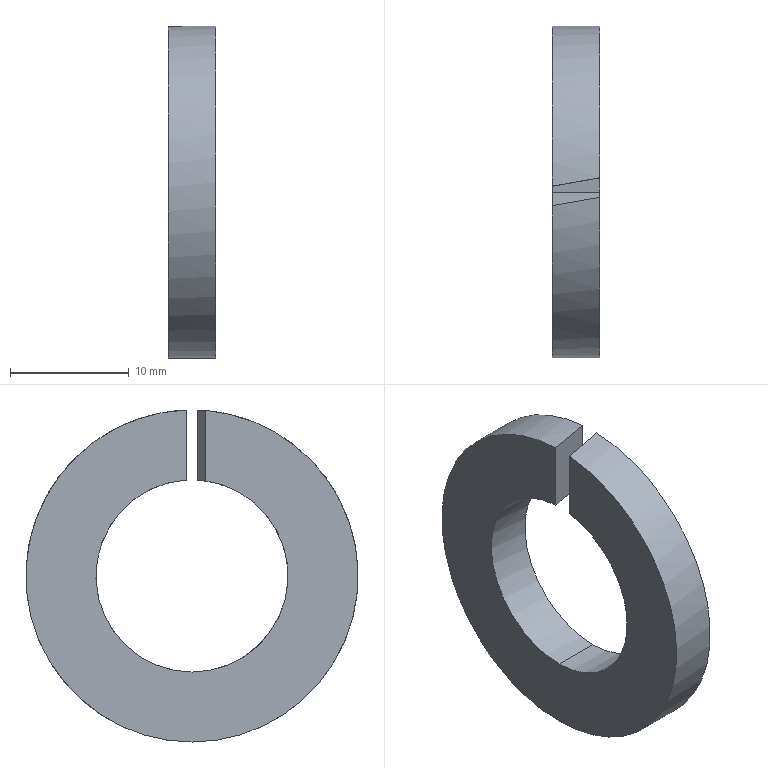Part | STEP file | 0229_320_SSLW16 | 1 solid | 8 faces | box 4 x 28 x 27.992 mm | volume 1600 mm3 | cylinder 4 | plane 4 | commonest cylinder face diameters 16.2 x2 28 x2
STEP:
#1=CARTESIAN_POINT('',(0.,0.,0.));
#2=DIRECTION('',(0.,0.,1.));
#3=DIRECTION('',(1.,0.,0.));
#4=AXIS2_PLACEMENT_3D('',#1,#2,#3);
#5=CARTESIAN_POINT('',(-2.,0.4698,8.086));
#6=VERTEX_POINT('',#5);
#7=CARTESIAN_POINT('',(2.,1.175,8.014));
#8=VERTEX_POINT('',#7);
#9=CARTESIAN_POINT('',(-2.,0.4698,8.086));
#10=CARTESIAN_POINT('',(-0.6611,0.7059,8.073));
#11=CARTESIAN_POINT('',(0.6731,0.9412,8.049));
#12=CARTESIAN_POINT('',(2.,1.175,8.014));
#13=(BOUNDED_CURVE()B_SPLINE_CURVE(3,(#9,#10,#11,#12),.UNSPECIFIED.,.F.,.F.)B_SPLINE_CURVE_WITH_KNOTS((4,4),(4.77,4.858),.PIECEWISE_BEZIER_KNOTS.)CURVE()GEOMETRIC_REPRESENTATION_ITEM()RATIONAL_B_SPLINE_CURVE((1.,0.9994,0.9994,1.))REPRESENTATION_ITEM(''));
#14=CARTESIAN_POINT('',(0.,0.,0.));
#15=DIRECTION('',(1.,0.,0.));
#16=DIRECTION('',(0.,0.,-1.));
#17=AXIS2_PLACEMENT_3D('',#14,#15,#16);
#18=CYLINDRICAL_SURFACE('',#17,8.1);
#19=CARTESIAN_POINT('',(3.084,-2.));
#20=CARTESIAN_POINT('',(3.082,-1.939));
#21=CARTESIAN_POINT('',(3.08,-1.818));
#22=CARTESIAN_POINT('',(3.076,-1.635));
#23=CARTESIAN_POINT('',(3.072,-1.453));
#24=CARTESIAN_POINT('',(3.068,-1.27));
#25=CARTESIAN_POINT('',(3.064,-1.088));
#26=CARTESIAN_POINT('',(3.06,-0.9059));
#27=CARTESIAN_POINT('',(3.056,-0.7237));
#28=CARTESIAN_POINT('',(3.052,-0.5415));
#29=CARTESIAN_POINT('',(3.048,-0.3595));
#30=CARTESIAN_POINT('',(3.044,-0.1775));
#31=CARTESIAN_POINT('',(3.04,0.004486));
#32=CARTESIAN_POINT('',(3.036,0.1864));
#33=CARTESIAN_POINT('',(3.032,0.3681));
#34=CARTESIAN_POINT('',(3.028,0.5499));
#35=CARTESIAN_POINT('',(3.024,0.7315));
#36=CARTESIAN_POINT('',(3.02,0.913));
#37=CARTESIAN_POINT('',(3.016,1.094));
#38=CARTESIAN_POINT('',(3.012,1.276));
#39=CARTESIAN_POINT('',(3.008,1.457));
#40=CARTESIAN_POINT('',(3.004,1.638));
#41=CARTESIAN_POINT('',(3.,1.819));
#42=CARTESIAN_POINT('',(2.997,1.94));
#43=CARTESIAN_POINT('',(2.996,2.));
#44=B_SPLINE_CURVE_WITH_KNOTS('',3,(#19,#20,#21,#22,#23,#24,#25,#26,#27,#28,#29,#30,#31,#32,#33,#34,#35,#36,#37,#38,#39,#40,#41,#42,#43),.UNSPECIFIED.,.F.,.F.,(4,1,1,1,1,1,1,1,1,1,1,1,1,1,1,1,1,1,1,1,1,1,4),(4.77,4.774,4.778,4.782,4.786,4.79,4.794,4.798,4.802,4.806,4.81,4.814,4.818,4.822,4.826,4.83,4.834,4.838,4.842,4.846,4.85,4.854,4.858),.QUASI_UNIFORM_KNOTS.);
#45=(GEOMETRIC_REPRESENTATION_CONTEXT(2)PARAMETRIC_REPRESENTATION_CONTEXT()REPRESENTATION_CONTEXT('',''));
#46=DEFINITIONAL_REPRESENTATION('',(#44),#45);
#47=PCURVE('',#18,#46);
#48=CARTESIAN_POINT('',(-4.08,0.1031,0.));
#49=DIRECTION('',(-0.1736,0.9848,0.));
#50=DIRECTION('',(-0.9848,-0.1736,0.));
#51=AXIS2_PLACEMENT_3D('',#48,#49,#50);
#52=PLANE('',#51);
#53=CARTESIAN_POINT('',(-2.112,8.086));
#54=CARTESIAN_POINT('',(-3.471,8.073));
#55=CARTESIAN_POINT('',(-4.826,8.049));
#56=CARTESIAN_POINT('',(-6.174,8.014));
#57=(BOUNDED_CURVE()B_SPLINE_CURVE(3,(#53,#54,#55,#56),.UNSPECIFIED.,.F.,.F.)B_SPLINE_CURVE_WITH_KNOTS((4,4),(4.77,4.858),.PIECEWISE_BEZIER_KNOTS.)CURVE()GEOMETRIC_REPRESENTATION_ITEM()RATIONAL_B_SPLINE_CURVE((1.,0.9994,0.9994,1.))REPRESENTATION_ITEM(''));
#58=(GEOMETRIC_REPRESENTATION_CONTEXT(2)PARAMETRIC_REPRESENTATION_CONTEXT()REPRESENTATION_CONTEXT('',''));
#59=DEFINITIONAL_REPRESENTATION('',(#57),#58);
#60=PCURVE('',#52,#59);
#61=SURFACE_CURVE('',#13,(#47,#60),.PCURVE_S1.);
#62=EDGE_CURVE('',#6,#8,#61,.T.);
#63=ORIENTED_EDGE('',*,*,#62,.T.);
#64=CARTESIAN_POINT('',(2.,0.,-8.1));
#65=VERTEX_POINT('',#64);
#66=CARTESIAN_POINT('',(2.,0.,0.));
#67=DIRECTION('',(-1.,0.,0.));
#68=DIRECTION('',(0.,0.,-1.));
#69=AXIS2_PLACEMENT_3D('',#66,#67,#68);
#70=CIRCLE('',#69,8.1);
#71=CARTESIAN_POINT('',(6.283,2.));
#72=DIRECTION('',(-1.,0.));
#73=VECTOR('',#72,1.);
#74=LINE('',#71,#73);
#75=(GEOMETRIC_REPRESENTATION_CONTEXT(2)PARAMETRIC_REPRESENTATION_CONTEXT()REPRESENTATION_CONTEXT('',''));
#76=DEFINITIONAL_REPRESENTATION('',(#74),#75);
#77=PCURVE('',#18,#76);
#78=CARTESIAN_POINT('',(2.,11.05,0.));
#79=DIRECTION('',(1.,0.,0.));
#80=DIRECTION('',(0.,0.,-1.));
#81=AXIS2_PLACEMENT_3D('',#78,#79,#80);
#82=PLANE('',#81);
#83=CARTESIAN_POINT('',(8.1,-11.05));
#84=CARTESIAN_POINT('',(8.1,-25.08));
#85=CARTESIAN_POINT('',(-4.05,-18.065));
#86=CARTESIAN_POINT('',(-16.2,-11.05));
#87=CARTESIAN_POINT('',(-4.05,-4.035));
#88=CARTESIAN_POINT('',(8.1,2.98));
#89=CARTESIAN_POINT('',(8.1,-11.05));
#90=(BOUNDED_CURVE()B_SPLINE_CURVE(2,(#83,#84,#85,#86,#87,#88,#89),.UNSPECIFIED.,.T.,.F.)B_SPLINE_CURVE_WITH_KNOTS((1,2,2,2,2,1),(-2.094,0.,2.094,4.189,6.283,8.378),.UNSPECIFIED.)CURVE()GEOMETRIC_REPRESENTATION_ITEM()RATIONAL_B_SPLINE_CURVE((1.,0.5,1.,0.5,1.,0.5,1.))REPRESENTATION_ITEM(''));
#91=(GEOMETRIC_REPRESENTATION_CONTEXT(2)PARAMETRIC_REPRESENTATION_CONTEXT()REPRESENTATION_CONTEXT('',''));
#92=DEFINITIONAL_REPRESENTATION('',(#90),#91);
#93=PCURVE('',#82,#92);
#94=SURFACE_CURVE('',#70,(#77,#93),.PCURVE_S1.);
#95=EDGE_CURVE('',#8,#65,#94,.T.);
#96=ORIENTED_EDGE('',*,*,#95,.T.);
#97=CARTESIAN_POINT('',(-2.,0.,-8.1));
#98=VERTEX_POINT('',#97);
#99=CARTESIAN_POINT('',(0.,0.,-8.1));
#100=DIRECTION('',(1.,0.,0.));
#101=VECTOR('',#100,1.);
#102=LINE('',#99,#101);
#103=CARTESIAN_POINT('',(0.,0.));
#104=DIRECTION('',(0.,1.));
#105=VECTOR('',#104,1.);
#106=LINE('',#103,#105);
#107=(GEOMETRIC_REPRESENTATION_CONTEXT(2)PARAMETRIC_REPRESENTATION_CONTEXT()REPRESENTATION_CONTEXT('',''));
#108=DEFINITIONAL_REPRESENTATION('',(#106),#107);
#109=PCURVE('',#18,#108);
#110=CARTESIAN_POINT('',(0.,0.,0.));
#111=DIRECTION('',(1.,0.,0.));
#112=DIRECTION('',(0.,0.,-1.));
#113=AXIS2_PLACEMENT_3D('',#110,#111,#112);
#114=CYLINDRICAL_SURFACE('',#113,8.1);
#115=CARTESIAN_POINT('',(6.283,0.));
#116=DIRECTION('',(0.,1.));
#117=VECTOR('',#116,1.);
#118=LINE('',#115,#117);
#119=(GEOMETRIC_REPRESENTATION_CONTEXT(2)PARAMETRIC_REPRESENTATION_CONTEXT()REPRESENTATION_CONTEXT('',''));
#120=DEFINITIONAL_REPRESENTATION('',(#118),#119);
#121=PCURVE('',#114,#120);
#122=SURFACE_CURVE('',#102,(#109,#121),.PCURVE_S1.);
#123=EDGE_CURVE('',#98,#65,#122,.T.);
#124=ORIENTED_EDGE('',*,*,#123,.F.);
#125=CARTESIAN_POINT('',(-2.,0.,0.));
#126=DIRECTION('',(1.,0.,0.));
#127=DIRECTION('',(0.,0.,-1.));
#128=AXIS2_PLACEMENT_3D('',#125,#126,#127);
#129=CIRCLE('',#128,8.1);
#130=CARTESIAN_POINT('',(0.,-2.));
#131=DIRECTION('',(1.,0.));
#132=VECTOR('',#131,1.);
#133=LINE('',#130,#132);
#134=(GEOMETRIC_REPRESENTATION_CONTEXT(2)PARAMETRIC_REPRESENTATION_CONTEXT()REPRESENTATION_CONTEXT('',''));
#135=DEFINITIONAL_REPRESENTATION('',(#133),#134);
#136=PCURVE('',#18,#135);
#137=CARTESIAN_POINT('',(-2.,11.05,0.));
#138=DIRECTION('',(-1.,0.,0.));
#139=DIRECTION('',(0.,0.,1.));
#140=AXIS2_PLACEMENT_3D('',#137,#138,#139);
#141=PLANE('',#140);
#142=CARTESIAN_POINT('',(-8.1,-11.05));
#143=CARTESIAN_POINT('',(-8.1,2.98));
#144=CARTESIAN_POINT('',(4.05,-4.035));
#145=CARTESIAN_POINT('',(16.2,-11.05));
#146=CARTESIAN_POINT('',(4.05,-18.065));
#147=CARTESIAN_POINT('',(-8.1,-25.08));
#148=CARTESIAN_POINT('',(-8.1,-11.05));
#149=(BOUNDED_CURVE()B_SPLINE_CURVE(2,(#142,#143,#144,#145,#146,#147,#148),.UNSPECIFIED.,.T.,.F.)B_SPLINE_CURVE_WITH_KNOTS((1,2,2,2,2,1),(-2.094,0.,2.094,4.189,6.283,8.378),.UNSPECIFIED.)CURVE()GEOMETRIC_REPRESENTATION_ITEM()RATIONAL_B_SPLINE_CURVE((1.,0.5,1.,0.5,1.,0.5,1.))REPRESENTATION_ITEM(''));
#150=(GEOMETRIC_REPRESENTATION_CONTEXT(2)PARAMETRIC_REPRESENTATION_CONTEXT()REPRESENTATION_CONTEXT('',''));
#151=DEFINITIONAL_REPRESENTATION('',(#149),#150);
#152=PCURVE('',#141,#151);
#153=SURFACE_CURVE('',#129,(#136,#152),.PCURVE_S1.);
#154=EDGE_CURVE('',#98,#6,#153,.T.);
#155=ORIENTED_EDGE('',*,*,#154,.T.);
#156=EDGE_LOOP('',(#63,#96,#124,#155));
#157=FACE_BOUND('',#156,.F.);
#158=ADVANCED_FACE('',(#157),#18,.F.);
#159=CARTESIAN_POINT('',(-2.,0.,-14.));
#160=VERTEX_POINT('',#159);
#161=CARTESIAN_POINT('',(-2.,-1.175,13.951));
#162=VERTEX_POINT('',#161);
#163=CARTESIAN_POINT('',(-2.,0.,0.));
#164=DIRECTION('',(-1.,0.,0.));
#165=DIRECTION('',(0.,0.,-1.));
#166=AXIS2_PLACEMENT_3D('',#163,#164,#165);
#167=CIRCLE('',#166,14.);
#168=CARTESIAN_POINT('',(0.,0.,0.));
#169=DIRECTION('',(1.,0.,0.));
#170=DIRECTION('',(0.,0.,-1.));
#171=AXIS2_PLACEMENT_3D('',#168,#169,#170);
#172=CYLINDRICAL_SURFACE('',#171,14.);
#173=CARTESIAN_POINT('',(6.283,-2.));
#174=DIRECTION('',(-1.,0.));
#175=VECTOR('',#174,1.);
#176=LINE('',#173,#175);
#177=(GEOMETRIC_REPRESENTATION_CONTEXT(2)PARAMETRIC_REPRESENTATION_CONTEXT()REPRESENTATION_CONTEXT('',''));
#178=DEFINITIONAL_REPRESENTATION('',(#176),#177);
#179=PCURVE('',#172,#178);
#180=CARTESIAN_POINT('',(0.,-11.05));
#181=DIRECTION('',(-1.,0.));
#182=AXIS2_PLACEMENT_2D('',#180,#181);
#183=CIRCLE('',#182,14.);
#184=(GEOMETRIC_REPRESENTATION_CONTEXT(2)PARAMETRIC_REPRESENTATION_CONTEXT()REPRESENTATION_CONTEXT('',''));
#185=DEFINITIONAL_REPRESENTATION('',(#183),#184);
#186=PCURVE('',#141,#185);
#187=SURFACE_CURVE('',#167,(#179,#186),.PCURVE_S1.);
#188=EDGE_CURVE('',#160,#162,#187,.T.);
#189=ORIENTED_EDGE('',*,*,#188,.F.);
#190=CARTESIAN_POINT('',(2.,0.,-14.));
#191=VERTEX_POINT('',#190);
#192=CARTESIAN_POINT('',(0.,0.,-14.));
#193=DIRECTION('',(1.,0.,0.));
#194=VECTOR('',#193,1.);
#195=LINE('',#192,#194);
#196=CARTESIAN_POINT('',(6.283,0.));
#197=DIRECTION('',(0.,1.));
#198=VECTOR('',#197,1.);
#199=LINE('',#196,#198);
#200=(GEOMETRIC_REPRESENTATION_CONTEXT(2)PARAMETRIC_REPRESENTATION_CONTEXT()REPRESENTATION_CONTEXT('',''));
#201=DEFINITIONAL_REPRESENTATION('',(#199),#200);
#202=PCURVE('',#172,#201);
#203=CARTESIAN_POINT('',(0.,0.,0.));
#204=DIRECTION('',(1.,0.,0.));
#205=DIRECTION('',(0.,0.,-1.));
#206=AXIS2_PLACEMENT_3D('',#203,#204,#205);
#207=CYLINDRICAL_SURFACE('',#206,14.);
#208=CARTESIAN_POINT('',(0.,0.));
#209=DIRECTION('',(0.,1.));
#210=VECTOR('',#209,1.);
#211=LINE('',#208,#210);
#212=(GEOMETRIC_REPRESENTATION_CONTEXT(2)PARAMETRIC_REPRESENTATION_CONTEXT()REPRESENTATION_CONTEXT('',''));
#213=DEFINITIONAL_REPRESENTATION('',(#211),#212);
#214=PCURVE('',#207,#213);
#215=SURFACE_CURVE('',#195,(#202,#214),.PCURVE_S1.);
#216=EDGE_CURVE('',#160,#191,#215,.T.);
#217=ORIENTED_EDGE('',*,*,#216,.T.);
#218=CARTESIAN_POINT('',(2.,-0.4698,13.992));
#219=VERTEX_POINT('',#218);
#220=CARTESIAN_POINT('',(2.,0.,0.));
#221=DIRECTION('',(-1.,0.,0.));
#222=DIRECTION('',(0.,0.,-1.));
#223=AXIS2_PLACEMENT_3D('',#220,#221,#222);
#224=CIRCLE('',#223,14.);
#225=CARTESIAN_POINT('',(6.283,2.));
#226=DIRECTION('',(-1.,0.));
#227=VECTOR('',#226,1.);
#228=LINE('',#225,#227);
#229=(GEOMETRIC_REPRESENTATION_CONTEXT(2)PARAMETRIC_REPRESENTATION_CONTEXT()REPRESENTATION_CONTEXT('',''));
#230=DEFINITIONAL_REPRESENTATION('',(#228),#229);
#231=PCURVE('',#172,#230);
#232=CARTESIAN_POINT('',(14.,-11.05));
#233=CARTESIAN_POINT('',(14.,-35.299));
#234=CARTESIAN_POINT('',(-7.,-23.174));
#235=CARTESIAN_POINT('',(-28.,-11.05));
#236=CARTESIAN_POINT('',(-7.,1.074));
#237=CARTESIAN_POINT('',(14.,13.199));
#238=CARTESIAN_POINT('',(14.,-11.05));
#239=(BOUNDED_CURVE()B_SPLINE_CURVE(2,(#232,#233,#234,#235,#236,#237,#238),.UNSPECIFIED.,.T.,.F.)B_SPLINE_CURVE_WITH_KNOTS((1,2,2,2,2,1),(-2.094,0.,2.094,4.189,6.283,8.378),.UNSPECIFIED.)CURVE()GEOMETRIC_REPRESENTATION_ITEM()RATIONAL_B_SPLINE_CURVE((1.,0.5,1.,0.5,1.,0.5,1.))REPRESENTATION_ITEM(''));
#240=(GEOMETRIC_REPRESENTATION_CONTEXT(2)PARAMETRIC_REPRESENTATION_CONTEXT()REPRESENTATION_CONTEXT('',''));
#241=DEFINITIONAL_REPRESENTATION('',(#239),#240);
#242=PCURVE('',#82,#241);
#243=SURFACE_CURVE('',#224,(#231,#242),.PCURVE_S1.);
#244=EDGE_CURVE('',#191,#219,#243,.T.);
#245=ORIENTED_EDGE('',*,*,#244,.T.);
#246=CARTESIAN_POINT('',(2.,-0.4698,13.992));
#247=CARTESIAN_POINT('',(0.6648,-0.7053,13.984));
#248=CARTESIAN_POINT('',(-0.6688,-0.9404,13.97));
#249=CARTESIAN_POINT('',(-2.,-1.175,13.951));
#250=(BOUNDED_CURVE()B_SPLINE_CURVE(3,(#246,#247,#248,#249),.UNSPECIFIED.,.F.,.F.)B_SPLINE_CURVE_WITH_KNOTS((4,4),(1.604,1.655),.PIECEWISE_BEZIER_KNOTS.)CURVE()GEOMETRIC_REPRESENTATION_ITEM()RATIONAL_B_SPLINE_CURVE((1.,0.9998,0.9998,1.))REPRESENTATION_ITEM(''));
#251=CARTESIAN_POINT('',(3.175,2.));
#252=CARTESIAN_POINT('',(3.176,1.939));
#253=CARTESIAN_POINT('',(3.177,1.818));
#254=CARTESIAN_POINT('',(3.18,1.636));
#255=CARTESIAN_POINT('',(3.182,1.454));
#256=CARTESIAN_POINT('',(3.184,1.272));
#257=CARTESIAN_POINT('',(3.187,1.09));
#258=CARTESIAN_POINT('',(3.189,0.908));
#259=CARTESIAN_POINT('',(3.191,0.7261));
#260=CARTESIAN_POINT('',(3.194,0.5442));
#261=CARTESIAN_POINT('',(3.196,0.3623));
#262=CARTESIAN_POINT('',(3.198,0.1804));
#263=CARTESIAN_POINT('',(3.2,-0.00149));
#264=CARTESIAN_POINT('',(3.203,-0.1833));
#265=CARTESIAN_POINT('',(3.205,-0.3651));
#266=CARTESIAN_POINT('',(3.207,-0.5469));
#267=CARTESIAN_POINT('',(3.21,-0.7287));
#268=CARTESIAN_POINT('',(3.212,-0.9104));
#269=CARTESIAN_POINT('',(3.214,-1.092));
#270=CARTESIAN_POINT('',(3.216,-1.274));
#271=CARTESIAN_POINT('',(3.219,-1.455));
#272=CARTESIAN_POINT('',(3.221,-1.637));
#273=CARTESIAN_POINT('',(3.223,-1.818));
#274=CARTESIAN_POINT('',(3.225,-1.94));
#275=CARTESIAN_POINT('',(3.226,-2.));
#276=B_SPLINE_CURVE_WITH_KNOTS('',3,(#251,#252,#253,#254,#255,#256,#257,#258,#259,#260,#261,#262,#263,#264,#265,#266,#267,#268,#269,#270,#271,#272,#273,#274,#275),.UNSPECIFIED.,.F.,.F.,(4,1,1,1,1,1,1,1,1,1,1,1,1,1,1,1,1,1,1,1,1,1,4),(1.604,1.607,1.609,1.611,1.614,1.616,1.618,1.62,1.623,1.625,1.627,1.63,1.632,1.634,1.636,1.639,1.641,1.643,1.646,1.648,1.65,1.653,1.655),.QUASI_UNIFORM_KNOTS.);
#277=(GEOMETRIC_REPRESENTATION_CONTEXT(2)PARAMETRIC_REPRESENTATION_CONTEXT()REPRESENTATION_CONTEXT('',''));
#278=DEFINITIONAL_REPRESENTATION('',(#276),#277);
#279=PCURVE('',#172,#278);
#280=CARTESIAN_POINT('',(4.08,-0.1031,0.));
#281=DIRECTION('',(0.1736,-0.9848,0.));
#282=DIRECTION('',(0.9848,0.1736,0.));
#283=AXIS2_PLACEMENT_3D('',#280,#281,#282);
#284=PLANE('',#283);
#285=CARTESIAN_POINT('',(-2.112,13.992));
#286=CARTESIAN_POINT('',(-3.468,13.984));
#287=CARTESIAN_POINT('',(-4.822,13.97));
#288=CARTESIAN_POINT('',(-6.174,13.951));
#289=(BOUNDED_CURVE()B_SPLINE_CURVE(3,(#285,#286,#287,#288),.UNSPECIFIED.,.F.,.F.)B_SPLINE_CURVE_WITH_KNOTS((4,4),(1.604,1.655),.PIECEWISE_BEZIER_KNOTS.)CURVE()GEOMETRIC_REPRESENTATION_ITEM()RATIONAL_B_SPLINE_CURVE((1.,0.9998,0.9998,1.))REPRESENTATION_ITEM(''));
#290=(GEOMETRIC_REPRESENTATION_CONTEXT(2)PARAMETRIC_REPRESENTATION_CONTEXT()REPRESENTATION_CONTEXT('',''));
#291=DEFINITIONAL_REPRESENTATION('',(#289),#290);
#292=PCURVE('',#284,#291);
#293=SURFACE_CURVE('',#250,(#279,#292),.PCURVE_S1.);
#294=EDGE_CURVE('',#219,#162,#293,.T.);
#295=ORIENTED_EDGE('',*,*,#294,.T.);
#296=EDGE_LOOP('',(#189,#217,#245,#295));
#297=FACE_BOUND('',#296,.T.);
#298=ADVANCED_FACE('',(#297),#172,.T.);
#299=CARTESIAN_POINT('',(-2.,-1.175,8.014));
#300=VERTEX_POINT('',#299);
#301=CARTESIAN_POINT('',(-2.,0.,0.));
#302=DIRECTION('',(1.,0.,0.));
#303=DIRECTION('',(0.,0.,-1.));
#304=AXIS2_PLACEMENT_3D('',#301,#302,#303);
#305=CIRCLE('',#304,8.1);
#306=CARTESIAN_POINT('',(-8.1,-11.05));
#307=CARTESIAN_POINT('',(-8.1,2.98));
#308=CARTESIAN_POINT('',(4.05,-4.035));
#309=CARTESIAN_POINT('',(16.2,-11.05));
#310=CARTESIAN_POINT('',(4.05,-18.065));
#311=CARTESIAN_POINT('',(-8.1,-25.08));
#312=CARTESIAN_POINT('',(-8.1,-11.05));
#313=(BOUNDED_CURVE()B_SPLINE_CURVE(2,(#306,#307,#308,#309,#310,#311,#312),.UNSPECIFIED.,.T.,.F.)B_SPLINE_CURVE_WITH_KNOTS((1,2,2,2,2,1),(-2.094,0.,2.094,4.189,6.283,8.378),.UNSPECIFIED.)CURVE()GEOMETRIC_REPRESENTATION_ITEM()RATIONAL_B_SPLINE_CURVE((1.,0.5,1.,0.5,1.,0.5,1.))REPRESENTATION_ITEM(''));
#314=(GEOMETRIC_REPRESENTATION_CONTEXT(2)PARAMETRIC_REPRESENTATION_CONTEXT()REPRESENTATION_CONTEXT('',''));
#315=DEFINITIONAL_REPRESENTATION('',(#313),#314);
#316=PCURVE('',#141,#315);
#317=CARTESIAN_POINT('',(0.,-2.));
#318=DIRECTION('',(1.,0.));
#319=VECTOR('',#318,1.);
#320=LINE('',#317,#319);
#321=(GEOMETRIC_REPRESENTATION_CONTEXT(2)PARAMETRIC_REPRESENTATION_CONTEXT()REPRESENTATION_CONTEXT('',''));
#322=DEFINITIONAL_REPRESENTATION('',(#320),#321);
#323=PCURVE('',#114,#322);
#324=SURFACE_CURVE('',#305,(#316,#323),.PCURVE_S1.);
#325=EDGE_CURVE('',#300,#98,#324,.T.);
#326=ORIENTED_EDGE('',*,*,#325,.T.);
#327=ORIENTED_EDGE('',*,*,#154,.T.);
#328=CARTESIAN_POINT('',(-2.,0.4698,13.992));
#329=VERTEX_POINT('',#328);
#330=CARTESIAN_POINT('',(-2.,0.4698,0.));
#331=DIRECTION('',(0.,0.,1.));
#332=VECTOR('',#331,1.);
#333=LINE('',#330,#332);
#334=CARTESIAN_POINT('',(0.,-10.58));
#335=DIRECTION('',(1.,0.));
#336=VECTOR('',#335,1.);
#337=LINE('',#334,#336);
#338=(GEOMETRIC_REPRESENTATION_CONTEXT(2)PARAMETRIC_REPRESENTATION_CONTEXT()REPRESENTATION_CONTEXT('',''));
#339=DEFINITIONAL_REPRESENTATION('',(#337),#338);
#340=PCURVE('',#141,#339);
#341=CARTESIAN_POINT('',(-2.112,0.));
#342=DIRECTION('',(0.,1.));
#343=VECTOR('',#342,1.);
#344=LINE('',#341,#343);
#345=(GEOMETRIC_REPRESENTATION_CONTEXT(2)PARAMETRIC_REPRESENTATION_CONTEXT()REPRESENTATION_CONTEXT('',''));
#346=DEFINITIONAL_REPRESENTATION('',(#344),#345);
#347=PCURVE('',#52,#346);
#348=SURFACE_CURVE('',#333,(#340,#347),.PCURVE_S1.);
#349=EDGE_CURVE('',#6,#329,#348,.T.);
#350=ORIENTED_EDGE('',*,*,#349,.T.);
#351=CARTESIAN_POINT('',(-2.,0.,0.));
#352=DIRECTION('',(-1.,0.,0.));
#353=DIRECTION('',(0.,0.,-1.));
#354=AXIS2_PLACEMENT_3D('',#351,#352,#353);
#355=CIRCLE('',#354,14.);
#356=CARTESIAN_POINT('',(0.,-11.05));
#357=DIRECTION('',(-1.,0.));
#358=AXIS2_PLACEMENT_2D('',#356,#357);
#359=CIRCLE('',#358,14.);
#360=(GEOMETRIC_REPRESENTATION_CONTEXT(2)PARAMETRIC_REPRESENTATION_CONTEXT()REPRESENTATION_CONTEXT('',''));
#361=DEFINITIONAL_REPRESENTATION('',(#359),#360);
#362=PCURVE('',#141,#361);
#363=CARTESIAN_POINT('',(6.283,-2.));
#364=DIRECTION('',(-1.,0.));
#365=VECTOR('',#364,1.);
#366=LINE('',#363,#365);
#367=(GEOMETRIC_REPRESENTATION_CONTEXT(2)PARAMETRIC_REPRESENTATION_CONTEXT()REPRESENTATION_CONTEXT('',''));
#368=DEFINITIONAL_REPRESENTATION('',(#366),#367);
#369=PCURVE('',#207,#368);
#370=SURFACE_CURVE('',#355,(#362,#369),.PCURVE_S1.);
#371=EDGE_CURVE('',#329,#160,#370,.T.);
#372=ORIENTED_EDGE('',*,*,#371,.T.);
#373=ORIENTED_EDGE('',*,*,#188,.T.);
#374=CARTESIAN_POINT('',(-2.,-1.175,0.));
#375=DIRECTION('',(0.,0.,-1.));
#376=VECTOR('',#375,1.);
#377=LINE('',#374,#376);
#378=CARTESIAN_POINT('',(0.,-12.225));
#379=DIRECTION('',(-1.,0.));
#380=VECTOR('',#379,1.);
#381=LINE('',#378,#380);
#382=(GEOMETRIC_REPRESENTATION_CONTEXT(2)PARAMETRIC_REPRESENTATION_CONTEXT()REPRESENTATION_CONTEXT('',''));
#383=DEFINITIONAL_REPRESENTATION('',(#381),#382);
#384=PCURVE('',#141,#383);
#385=CARTESIAN_POINT('',(-6.174,0.));
#386=DIRECTION('',(0.,-1.));
#387=VECTOR('',#386,1.);
#388=LINE('',#385,#387);
#389=(GEOMETRIC_REPRESENTATION_CONTEXT(2)PARAMETRIC_REPRESENTATION_CONTEXT()REPRESENTATION_CONTEXT('',''));
#390=DEFINITIONAL_REPRESENTATION('',(#388),#389);
#391=PCURVE('',#284,#390);
#392=SURFACE_CURVE('',#377,(#384,#391),.PCURVE_S1.);
#393=EDGE_CURVE('',#162,#300,#392,.T.);
#394=ORIENTED_EDGE('',*,*,#393,.T.);
#395=EDGE_LOOP('',(#326,#327,#350,#372,#373,#394));
#396=FACE_BOUND('',#395,.T.);
#397=ADVANCED_FACE('',(#396),#141,.T.);
#398=CARTESIAN_POINT('',(2.,-0.4698,8.086));
#399=VERTEX_POINT('',#398);
#400=CARTESIAN_POINT('',(2.,0.,0.));
#401=DIRECTION('',(-1.,0.,0.));
#402=DIRECTION('',(0.,0.,-1.));
#403=AXIS2_PLACEMENT_3D('',#400,#401,#402);
#404=CIRCLE('',#403,8.1);
#405=CARTESIAN_POINT('',(6.283,2.));
#406=DIRECTION('',(-1.,0.));
#407=VECTOR('',#406,1.);
#408=LINE('',#405,#407);
#409=(GEOMETRIC_REPRESENTATION_CONTEXT(2)PARAMETRIC_REPRESENTATION_CONTEXT()REPRESENTATION_CONTEXT('',''));
#410=DEFINITIONAL_REPRESENTATION('',(#408),#409);
#411=PCURVE('',#114,#410);
#412=CARTESIAN_POINT('',(8.1,-11.05));
#413=CARTESIAN_POINT('',(8.1,-25.08));
#414=CARTESIAN_POINT('',(-4.05,-18.065));
#415=CARTESIAN_POINT('',(-16.2,-11.05));
#416=CARTESIAN_POINT('',(-4.05,-4.035));
#417=CARTESIAN_POINT('',(8.1,2.98));
#418=CARTESIAN_POINT('',(8.1,-11.05));
#419=(BOUNDED_CURVE()B_SPLINE_CURVE(2,(#412,#413,#414,#415,#416,#417,#418),.UNSPECIFIED.,.T.,.F.)B_SPLINE_CURVE_WITH_KNOTS((1,2,2,2,2,1),(-2.094,0.,2.094,4.189,6.283,8.378),.UNSPECIFIED.)CURVE()GEOMETRIC_REPRESENTATION_ITEM()RATIONAL_B_SPLINE_CURVE((1.,0.5,1.,0.5,1.,0.5,1.))REPRESENTATION_ITEM(''));
#420=(GEOMETRIC_REPRESENTATION_CONTEXT(2)PARAMETRIC_REPRESENTATION_CONTEXT()REPRESENTATION_CONTEXT('',''));
#421=DEFINITIONAL_REPRESENTATION('',(#419),#420);
#422=PCURVE('',#82,#421);
#423=SURFACE_CURVE('',#404,(#411,#422),.PCURVE_S1.);
#424=EDGE_CURVE('',#65,#399,#423,.T.);
#425=ORIENTED_EDGE('',*,*,#424,.T.);
#426=CARTESIAN_POINT('',(2.,-0.4698,8.086));
#427=CARTESIAN_POINT('',(0.6611,-0.7059,8.073));
#428=CARTESIAN_POINT('',(-0.6731,-0.9412,8.049));
#429=CARTESIAN_POINT('',(-2.,-1.175,8.014));
#430=(BOUNDED_CURVE()B_SPLINE_CURVE(3,(#426,#427,#428,#429),.UNSPECIFIED.,.F.,.F.)B_SPLINE_CURVE_WITH_KNOTS((4,4),(1.629,1.716),.PIECEWISE_BEZIER_KNOTS.)CURVE()GEOMETRIC_REPRESENTATION_ITEM()RATIONAL_B_SPLINE_CURVE((1.,0.9994,0.9994,1.))REPRESENTATION_ITEM(''));
#431=CARTESIAN_POINT('',(3.2,2.));
#432=CARTESIAN_POINT('',(3.201,1.939));
#433=CARTESIAN_POINT('',(3.204,1.818));
#434=CARTESIAN_POINT('',(3.208,1.635));
#435=CARTESIAN_POINT('',(3.212,1.453));
#436=CARTESIAN_POINT('',(3.216,1.27));
#437=CARTESIAN_POINT('',(3.22,1.088));
#438=CARTESIAN_POINT('',(3.224,0.9059));
#439=CARTESIAN_POINT('',(3.227,0.7237));
#440=CARTESIAN_POINT('',(3.231,0.5415));
#441=CARTESIAN_POINT('',(3.235,0.3595));
#442=CARTESIAN_POINT('',(3.239,0.1775));
#443=CARTESIAN_POINT('',(3.243,-0.004486));
#444=CARTESIAN_POINT('',(3.247,-0.1864));
#445=CARTESIAN_POINT('',(3.251,-0.3681));
#446=CARTESIAN_POINT('',(3.255,-0.5499));
#447=CARTESIAN_POINT('',(3.259,-0.7315));
#448=CARTESIAN_POINT('',(3.263,-0.913));
#449=CARTESIAN_POINT('',(3.267,-1.094));
#450=CARTESIAN_POINT('',(3.271,-1.276));
#451=CARTESIAN_POINT('',(3.275,-1.457));
#452=CARTESIAN_POINT('',(3.279,-1.638));
#453=CARTESIAN_POINT('',(3.283,-1.819));
#454=CARTESIAN_POINT('',(3.286,-1.94));
#455=CARTESIAN_POINT('',(3.287,-2.));
#456=B_SPLINE_CURVE_WITH_KNOTS('',3,(#431,#432,#433,#434,#435,#436,#437,#438,#439,#440,#441,#442,#443,#444,#445,#446,#447,#448,#449,#450,#451,#452,#453,#454,#455),.UNSPECIFIED.,.F.,.F.,(4,1,1,1,1,1,1,1,1,1,1,1,1,1,1,1,1,1,1,1,1,1,4),(1.629,1.633,1.637,1.641,1.645,1.649,1.653,1.657,1.661,1.665,1.669,1.673,1.677,1.681,1.685,1.689,1.693,1.696,1.7,1.704,1.708,1.712,1.716),.QUASI_UNIFORM_KNOTS.);
#457=(GEOMETRIC_REPRESENTATION_CONTEXT(2)PARAMETRIC_REPRESENTATION_CONTEXT()REPRESENTATION_CONTEXT('',''));
#458=DEFINITIONAL_REPRESENTATION('',(#456),#457);
#459=PCURVE('',#114,#458);
#460=CARTESIAN_POINT('',(-2.112,8.086));
#461=CARTESIAN_POINT('',(-3.471,8.073));
#462=CARTESIAN_POINT('',(-4.826,8.049));
#463=CARTESIAN_POINT('',(-6.174,8.014));
#464=(BOUNDED_CURVE()B_SPLINE_CURVE(3,(#460,#461,#462,#463),.UNSPECIFIED.,.F.,.F.)B_SPLINE_CURVE_WITH_KNOTS((4,4),(1.629,1.716),.PIECEWISE_BEZIER_KNOTS.)CURVE()GEOMETRIC_REPRESENTATION_ITEM()RATIONAL_B_SPLINE_CURVE((1.,0.9994,0.9994,1.))REPRESENTATION_ITEM(''));
#465=(GEOMETRIC_REPRESENTATION_CONTEXT(2)PARAMETRIC_REPRESENTATION_CONTEXT()REPRESENTATION_CONTEXT('',''));
#466=DEFINITIONAL_REPRESENTATION('',(#464),#465);
#467=PCURVE('',#284,#466);
#468=SURFACE_CURVE('',#430,(#459,#467),.PCURVE_S1.);
#469=EDGE_CURVE('',#399,#300,#468,.T.);
#470=ORIENTED_EDGE('',*,*,#469,.T.);
#471=ORIENTED_EDGE('',*,*,#325,.T.);
#472=ORIENTED_EDGE('',*,*,#123,.T.);
#473=EDGE_LOOP('',(#425,#470,#471,#472));
#474=FACE_BOUND('',#473,.F.);
#475=ADVANCED_FACE('',(#474),#114,.F.);
#476=ORIENTED_EDGE('',*,*,#469,.T.);
#477=ORIENTED_EDGE('',*,*,#393,.F.);
#478=ORIENTED_EDGE('',*,*,#294,.F.);
#479=CARTESIAN_POINT('',(2.,-0.4698,0.));
#480=DIRECTION('',(0.,0.,1.));
#481=VECTOR('',#480,1.);
#482=LINE('',#479,#481);
#483=CARTESIAN_POINT('',(-2.112,0.));
#484=DIRECTION('',(0.,1.));
#485=VECTOR('',#484,1.);
#486=LINE('',#483,#485);
#487=(GEOMETRIC_REPRESENTATION_CONTEXT(2)PARAMETRIC_REPRESENTATION_CONTEXT()REPRESENTATION_CONTEXT('',''));
#488=DEFINITIONAL_REPRESENTATION('',(#486),#487);
#489=PCURVE('',#284,#488);
#490=CARTESIAN_POINT('',(0.,-11.52));
#491=DIRECTION('',(-1.,0.));
#492=VECTOR('',#491,1.);
#493=LINE('',#490,#492);
#494=(GEOMETRIC_REPRESENTATION_CONTEXT(2)PARAMETRIC_REPRESENTATION_CONTEXT()REPRESENTATION_CONTEXT('',''));
#495=DEFINITIONAL_REPRESENTATION('',(#493),#494);
#496=PCURVE('',#82,#495);
#497=SURFACE_CURVE('',#482,(#489,#496),.PCURVE_S1.);
#498=EDGE_CURVE('',#399,#219,#497,.T.);
#499=ORIENTED_EDGE('',*,*,#498,.F.);
#500=EDGE_LOOP('',(#476,#477,#478,#499));
#501=FACE_BOUND('',#500,.T.);
#502=ADVANCED_FACE('',(#501),#284,.F.);
#503=ORIENTED_EDGE('',*,*,#216,.F.);
#504=ORIENTED_EDGE('',*,*,#371,.F.);
#505=CARTESIAN_POINT('',(2.,1.175,13.951));
#506=VERTEX_POINT('',#505);
#507=CARTESIAN_POINT('',(-2.,0.4698,13.992));
#508=CARTESIAN_POINT('',(-0.6648,0.7053,13.984));
#509=CARTESIAN_POINT('',(0.6688,0.9404,13.97));
#510=CARTESIAN_POINT('',(2.,1.175,13.951));
#511=(BOUNDED_CURVE()B_SPLINE_CURVE(3,(#507,#508,#509,#510),.UNSPECIFIED.,.F.,.F.)B_SPLINE_CURVE_WITH_KNOTS((4,4),(4.746,4.796),.PIECEWISE_BEZIER_KNOTS.)CURVE()GEOMETRIC_REPRESENTATION_ITEM()RATIONAL_B_SPLINE_CURVE((1.,0.9998,0.9998,1.))REPRESENTATION_ITEM(''));
#512=CARTESIAN_POINT('',(3.108,-2.));
#513=CARTESIAN_POINT('',(3.107,-1.939));
#514=CARTESIAN_POINT('',(3.106,-1.818));
#515=CARTESIAN_POINT('',(3.103,-1.636));
#516=CARTESIAN_POINT('',(3.101,-1.454));
#517=CARTESIAN_POINT('',(3.099,-1.272));
#518=CARTESIAN_POINT('',(3.097,-1.09));
#519=CARTESIAN_POINT('',(3.094,-0.908));
#520=CARTESIAN_POINT('',(3.092,-0.7261));
#521=CARTESIAN_POINT('',(3.09,-0.5442));
#522=CARTESIAN_POINT('',(3.087,-0.3623));
#523=CARTESIAN_POINT('',(3.085,-0.1804));
#524=CARTESIAN_POINT('',(3.083,0.00149));
#525=CARTESIAN_POINT('',(3.08,0.1833));
#526=CARTESIAN_POINT('',(3.078,0.3651));
#527=CARTESIAN_POINT('',(3.076,0.5469));
#528=CARTESIAN_POINT('',(3.074,0.7287));
#529=CARTESIAN_POINT('',(3.071,0.9104));
#530=CARTESIAN_POINT('',(3.069,1.092));
#531=CARTESIAN_POINT('',(3.067,1.274));
#532=CARTESIAN_POINT('',(3.064,1.455));
#533=CARTESIAN_POINT('',(3.062,1.637));
#534=CARTESIAN_POINT('',(3.06,1.818));
#535=CARTESIAN_POINT('',(3.058,1.94));
#536=CARTESIAN_POINT('',(3.058,2.));
#537=B_SPLINE_CURVE_WITH_KNOTS('',3,(#512,#513,#514,#515,#516,#517,#518,#519,#520,#521,#522,#523,#524,#525,#526,#527,#528,#529,#530,#531,#532,#533,#534,#535,#536),.UNSPECIFIED.,.F.,.F.,(4,1,1,1,1,1,1,1,1,1,1,1,1,1,1,1,1,1,1,1,1,1,4),(4.746,4.748,4.751,4.753,4.755,4.757,4.76,4.762,4.764,4.767,4.769,4.771,4.773,4.776,4.778,4.78,4.783,4.785,4.787,4.79,4.792,4.794,4.796),.QUASI_UNIFORM_KNOTS.);
#538=(GEOMETRIC_REPRESENTATION_CONTEXT(2)PARAMETRIC_REPRESENTATION_CONTEXT()REPRESENTATION_CONTEXT('',''));
#539=DEFINITIONAL_REPRESENTATION('',(#537),#538);
#540=PCURVE('',#207,#539);
#541=CARTESIAN_POINT('',(-2.112,13.992));
#542=CARTESIAN_POINT('',(-3.468,13.984));
#543=CARTESIAN_POINT('',(-4.822,13.97));
#544=CARTESIAN_POINT('',(-6.174,13.951));
#545=(BOUNDED_CURVE()B_SPLINE_CURVE(3,(#541,#542,#543,#544),.UNSPECIFIED.,.F.,.F.)B_SPLINE_CURVE_WITH_KNOTS((4,4),(4.746,4.796),.PIECEWISE_BEZIER_KNOTS.)CURVE()GEOMETRIC_REPRESENTATION_ITEM()RATIONAL_B_SPLINE_CURVE((1.,0.9998,0.9998,1.))REPRESENTATION_ITEM(''));
#546=(GEOMETRIC_REPRESENTATION_CONTEXT(2)PARAMETRIC_REPRESENTATION_CONTEXT()REPRESENTATION_CONTEXT('',''));
#547=DEFINITIONAL_REPRESENTATION('',(#545),#546);
#548=PCURVE('',#52,#547);
#549=SURFACE_CURVE('',#511,(#540,#548),.PCURVE_S1.);
#550=EDGE_CURVE('',#329,#506,#549,.T.);
#551=ORIENTED_EDGE('',*,*,#550,.T.);
#552=CARTESIAN_POINT('',(2.,0.,0.));
#553=DIRECTION('',(-1.,0.,0.));
#554=DIRECTION('',(0.,0.,-1.));
#555=AXIS2_PLACEMENT_3D('',#552,#553,#554);
#556=CIRCLE('',#555,14.);
#557=CARTESIAN_POINT('',(6.283,2.));
#558=DIRECTION('',(-1.,0.));
#559=VECTOR('',#558,1.);
#560=LINE('',#557,#559);
#561=(GEOMETRIC_REPRESENTATION_CONTEXT(2)PARAMETRIC_REPRESENTATION_CONTEXT()REPRESENTATION_CONTEXT('',''));
#562=DEFINITIONAL_REPRESENTATION('',(#560),#561);
#563=PCURVE('',#207,#562);
#564=CARTESIAN_POINT('',(14.,-11.05));
#565=CARTESIAN_POINT('',(14.,-35.299));
#566=CARTESIAN_POINT('',(-7.,-23.174));
#567=CARTESIAN_POINT('',(-28.,-11.05));
#568=CARTESIAN_POINT('',(-7.,1.074));
#569=CARTESIAN_POINT('',(14.,13.199));
#570=CARTESIAN_POINT('',(14.,-11.05));
#571=(BOUNDED_CURVE()B_SPLINE_CURVE(2,(#564,#565,#566,#567,#568,#569,#570),.UNSPECIFIED.,.T.,.F.)B_SPLINE_CURVE_WITH_KNOTS((1,2,2,2,2,1),(-2.094,0.,2.094,4.189,6.283,8.378),.UNSPECIFIED.)CURVE()GEOMETRIC_REPRESENTATION_ITEM()RATIONAL_B_SPLINE_CURVE((1.,0.5,1.,0.5,1.,0.5,1.))REPRESENTATION_ITEM(''));
#572=(GEOMETRIC_REPRESENTATION_CONTEXT(2)PARAMETRIC_REPRESENTATION_CONTEXT()REPRESENTATION_CONTEXT('',''));
#573=DEFINITIONAL_REPRESENTATION('',(#571),#572);
#574=PCURVE('',#82,#573);
#575=SURFACE_CURVE('',#556,(#563,#574),.PCURVE_S1.);
#576=EDGE_CURVE('',#506,#191,#575,.T.);
#577=ORIENTED_EDGE('',*,*,#576,.T.);
#578=EDGE_LOOP('',(#503,#504,#551,#577));
#579=FACE_BOUND('',#578,.T.);
#580=ADVANCED_FACE('',(#579),#207,.T.);
#581=ORIENTED_EDGE('',*,*,#550,.F.);
#582=ORIENTED_EDGE('',*,*,#349,.F.);
#583=ORIENTED_EDGE('',*,*,#62,.T.);
#584=CARTESIAN_POINT('',(2.,1.175,0.));
#585=DIRECTION('',(0.,0.,-1.));
#586=VECTOR('',#585,1.);
#587=LINE('',#584,#586);
#588=CARTESIAN_POINT('',(-6.174,0.));
#589=DIRECTION('',(0.,-1.));
#590=VECTOR('',#589,1.);
#591=LINE('',#588,#590);
#592=(GEOMETRIC_REPRESENTATION_CONTEXT(2)PARAMETRIC_REPRESENTATION_CONTEXT()REPRESENTATION_CONTEXT('',''));
#593=DEFINITIONAL_REPRESENTATION('',(#591),#592);
#594=PCURVE('',#52,#593);
#595=CARTESIAN_POINT('',(0.,-9.875));
#596=DIRECTION('',(1.,0.));
#597=VECTOR('',#596,1.);
#598=LINE('',#595,#597);
#599=(GEOMETRIC_REPRESENTATION_CONTEXT(2)PARAMETRIC_REPRESENTATION_CONTEXT()REPRESENTATION_CONTEXT('',''));
#600=DEFINITIONAL_REPRESENTATION('',(#598),#599);
#601=PCURVE('',#82,#600);
#602=SURFACE_CURVE('',#587,(#594,#601),.PCURVE_S1.);
#603=EDGE_CURVE('',#506,#8,#602,.T.);
#604=ORIENTED_EDGE('',*,*,#603,.F.);
#605=EDGE_LOOP('',(#581,#582,#583,#604));
#606=FACE_BOUND('',#605,.T.);
#607=ADVANCED_FACE('',(#606),#52,.F.);
#608=ORIENTED_EDGE('',*,*,#576,.F.);
#609=ORIENTED_EDGE('',*,*,#603,.T.);
#610=ORIENTED_EDGE('',*,*,#95,.T.);
#611=ORIENTED_EDGE('',*,*,#424,.T.);
#612=ORIENTED_EDGE('',*,*,#498,.T.);
#613=ORIENTED_EDGE('',*,*,#244,.F.);
#614=EDGE_LOOP('',(#608,#609,#610,#611,#612,#613));
#615=FACE_BOUND('',#614,.T.);
#616=ADVANCED_FACE('',(#615),#82,.T.);
#617=CLOSED_SHELL('',(#158,#298,#397,#475,#502,#580,#607,#616));
#618=MANIFOLD_SOLID_BREP('',#617);
#619=(LENGTH_UNIT()NAMED_UNIT(*)SI_UNIT(.MILLI.,.METRE.));
#620=UNCERTAINTY_MEASURE_WITH_UNIT(LENGTH_MEASURE(0.0000001),#619,'','');
#621=(NAMED_UNIT(*)PLANE_ANGLE_UNIT()SI_UNIT($,.RADIAN.));
#622=(NAMED_UNIT(*)SI_UNIT($,.STERADIAN.)SOLID_ANGLE_UNIT());
#623=(GEOMETRIC_REPRESENTATION_CONTEXT(3)GLOBAL_UNCERTAINTY_ASSIGNED_CONTEXT((#620))GLOBAL_UNIT_ASSIGNED_CONTEXT((#619,#621,#622))REPRESENTATION_CONTEXT('',''));
#624=ADVANCED_BREP_SHAPE_REPRESENTATION('',(#4,#618),#623);